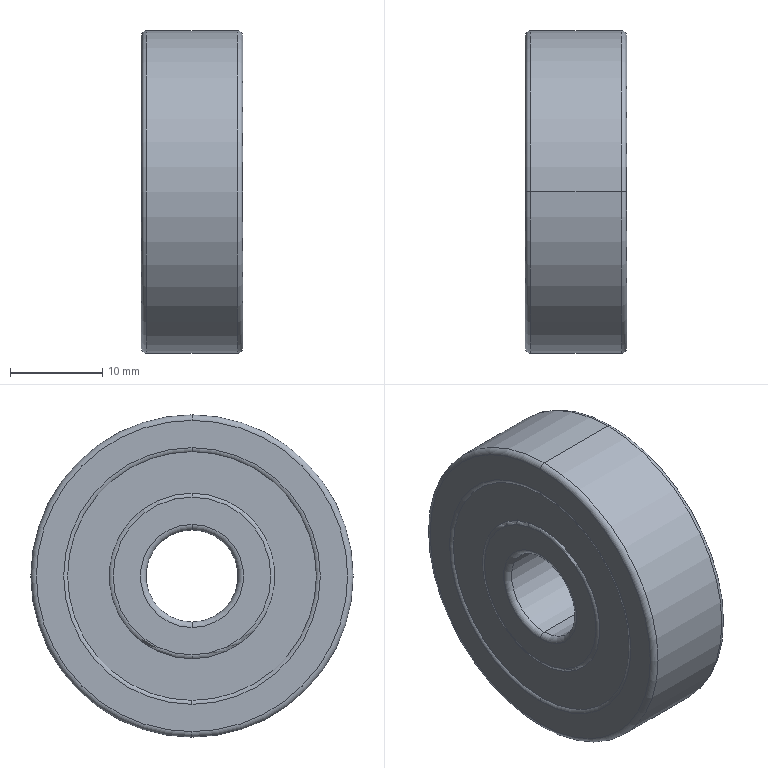Part | SolidWorks | features BaseBody 11 | 11 solids | 138 faces | box 11 x 35 x 35 mm | volume 7523 mm3 | cylinder 46 | sphere 40 | plane 26 | torus 26 | commonest cylinder face diameters 21.25 x17 23.75 x17 18.333 x4 26.667 x4 10 x2 35 x2